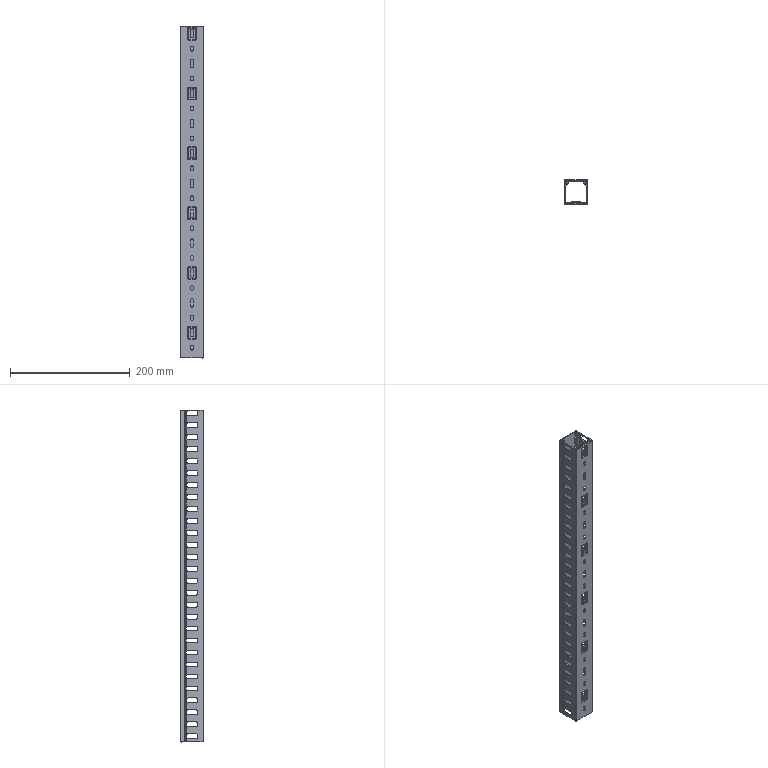Part | SolidWorks | features BaseBody 2 | 2 solids | 2211 faces | box 40 x 40.1 x 555 mm | volume 152024 mm3 | cylinder 1241 | plane 826 | sphere 96 | torus 48 | commonest cylinder face diameters 4 x224 1 x182 3.6 x174 3 x172 1.4 x171 1.464 x144